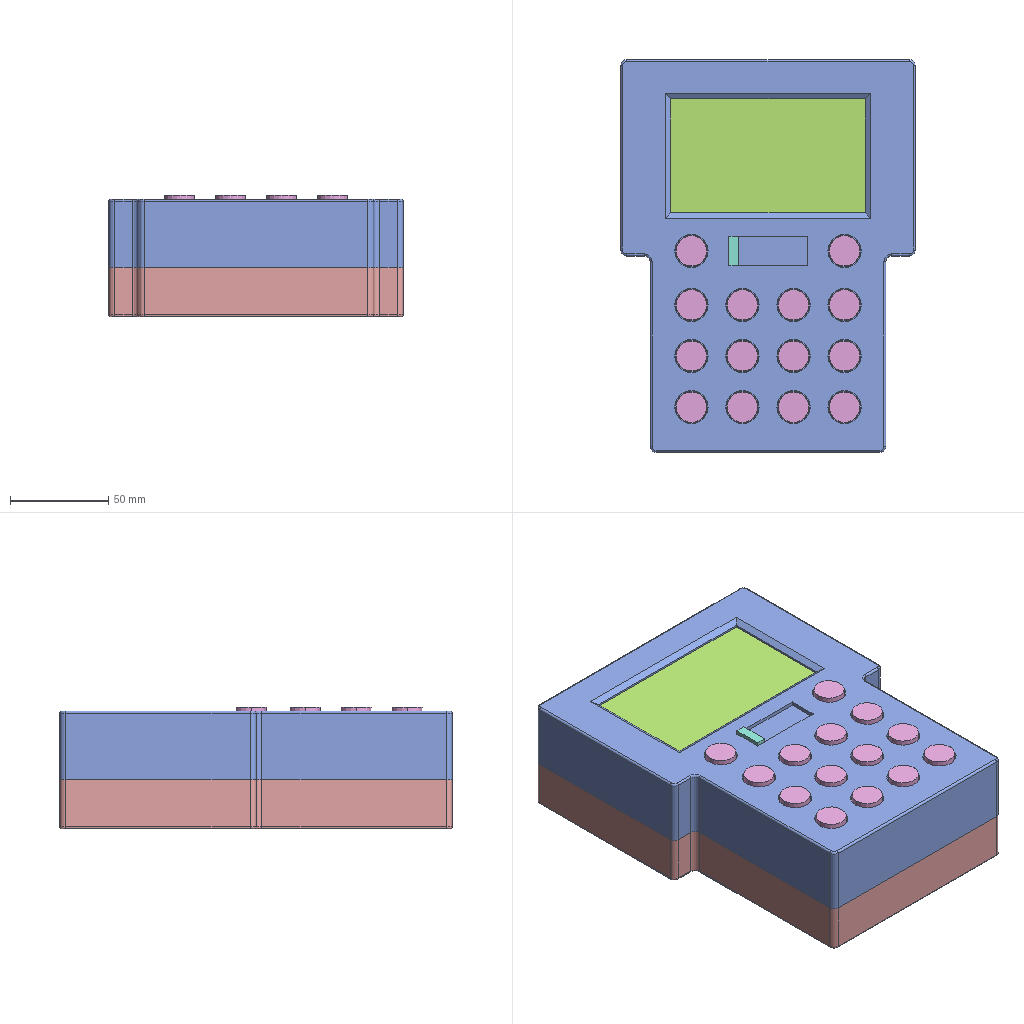Assembly | SolidWorks | 5 different items | 5 placed | box 150 x 200 x 62 mm
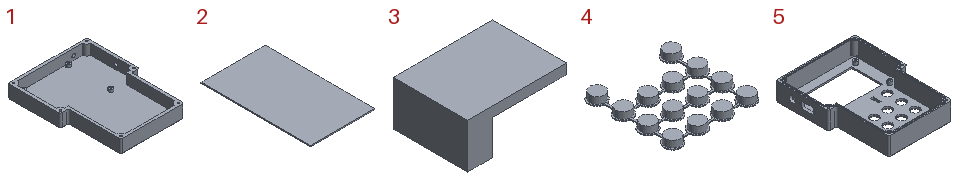Parts list (item | quantity | size | volume | features):
1 | x1 | 150 x 200 x 25 mm | 205338 mm3 | features ICE 7, Fillet 2, Extrusion 1
2 | x1 | 58 x 99 x 1 mm | 5742 mm3 | features Extrusion 1
3 | x1 | 20 x 15 x 9 mm | 1125 mm3 | features Extrusion 1, ICE 1
4 | x1 | 96 x 97.5 x 8 mm | 22308 mm3 | features Extrusion 1, ICE 1
5 | x1 | 150 x 200 x 35 mm | 192562 mm3 | features ICE 9, Fillet 2, Chamfer 1, Extrusion 1
Mates (type | each side: item.copy, entity, surface, feature):
Coincident | 1.1 face plane Boss-Extrude1 | 5.1 face plane Boss-Extrude1 | 3 times
Coincident | 5.1 face plane Boss-Extrude1 | 2.1 face plane Boss-Extrude1 | 2 times
DistanceDim | 2.1 face plane Boss-Extrude1 | 5.1 edge
Coincident | 5.1 face plane Cut-Extrude1 | 4.1 face plane Boss-Extrude1
Concentric | 5.1 face cylinder Boss-Extrude1 | 4.1 face cylinder Boss-Extrude2
Concentric | 5.1 face cylinder Cut-Extrude2 | 4.1 face cylinder Boss-Extrude2
Coincident | 5.1 face plane Cut-Extrude1 | 3.1 face plane Boss-Extrude2
Coincident | 5.1 face plane Cut-Extrude6 | 3.1 face plane Boss-Extrude1 | 2 times